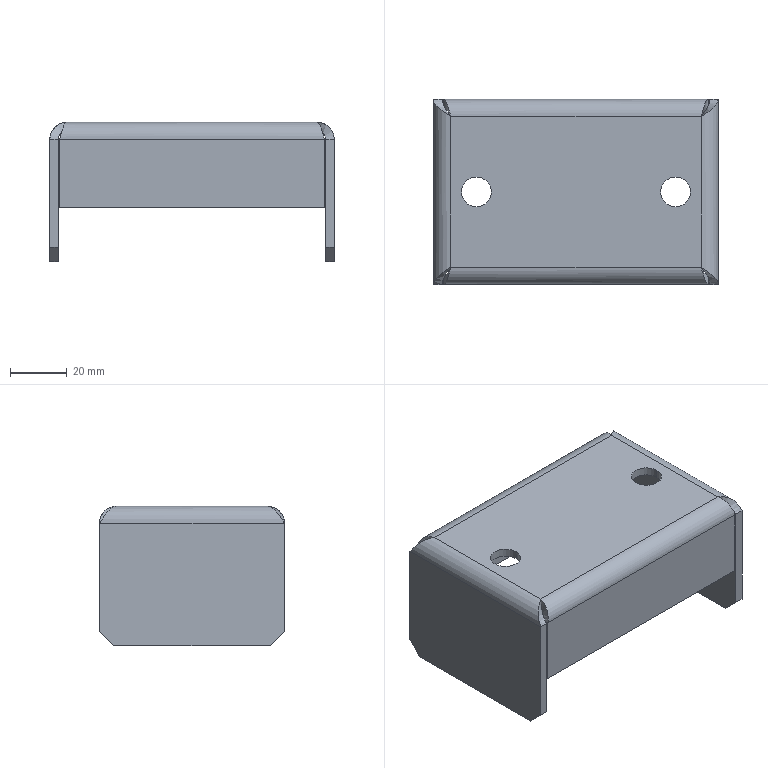Part | STEP file | SYL_0392D6J1SYL0380DJ1006-90462 | 1 solid | 46 faces | box 100 x 65 x 49 mm | volume 49825 mm3 | plane 26 | cylinder 12 | spline 8 | commonest cylinder face diameters 6 x4 10.5 x4 12 x4